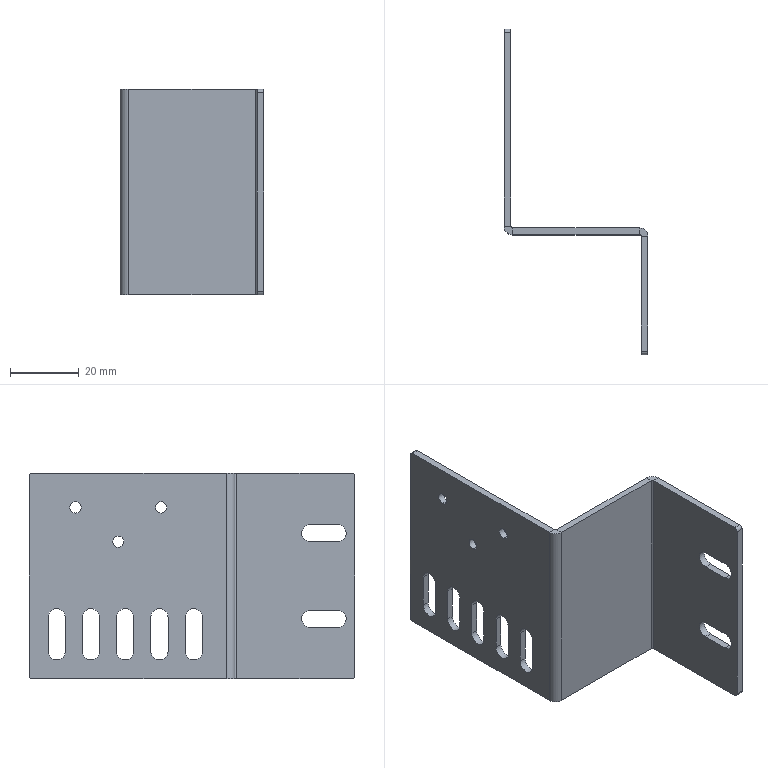Part | NX | features BREP 1 | 1 solid | 60 faces | box 42 x 95 x 60 mm | volume 15058 mm3 | plane 32 | cylinder 28 | commonest cylinder face diameters 5 x16 3.3 x6 2 x4 1 x2